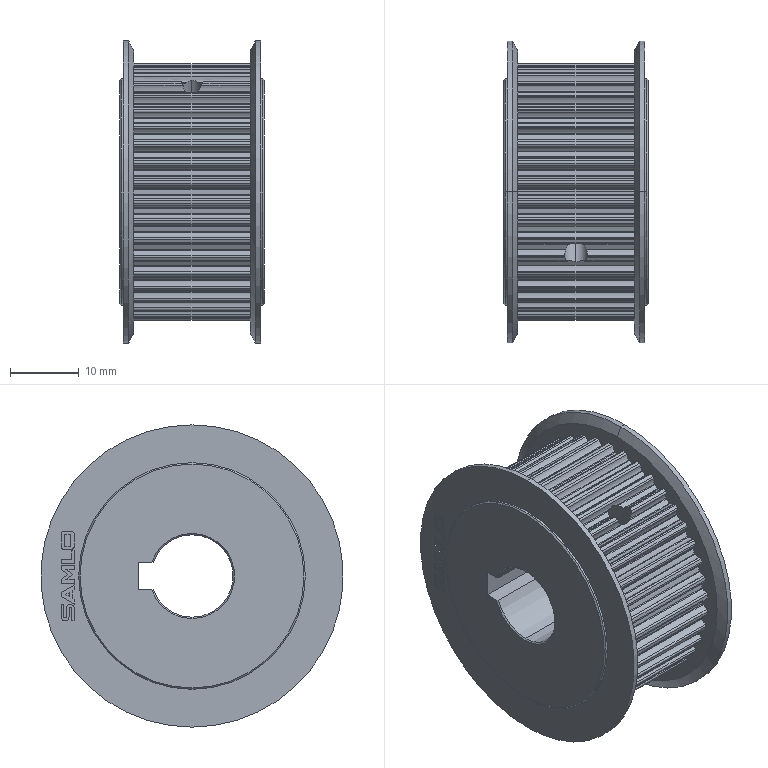Part | SolidWorks | features BaseBody 1 | 1 solid | 478 faces | box 21 x 44 x 44 mm | volume 20059 mm3 | cylinder 403 | plane 61 | cone 14 | commonest cylinder face diameters 0.56 x103 0.3 x97 3.95 x90 35.22 x43 37.44 x41 0.442 x4